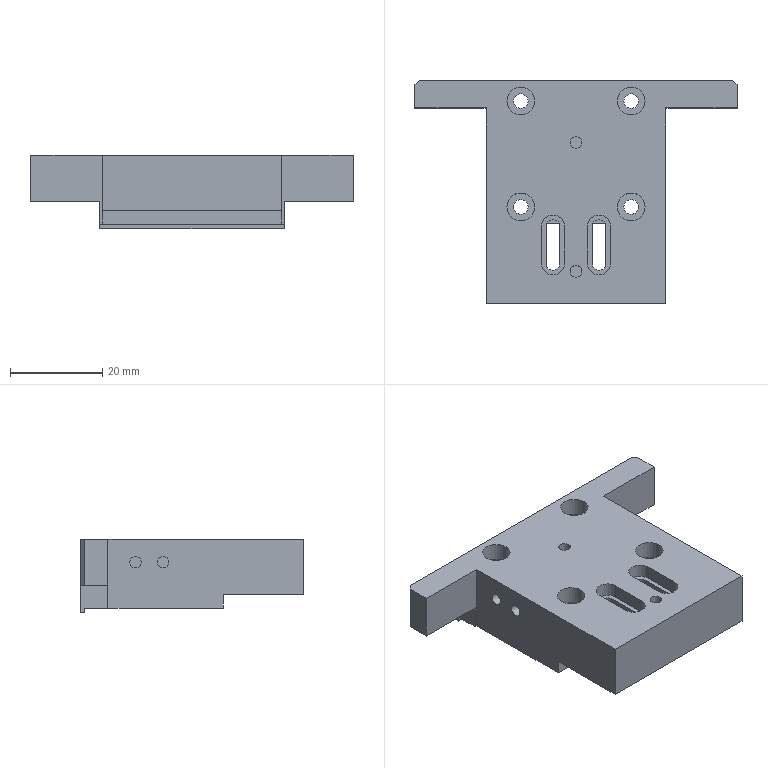NC program | NX | posted with a generic post | part box 70 x 48.5 x 16 mm
Whole program:
N10 G17 G21 G94 G90
(ADAPTIVE_MILLING , TOOL : D10)
N12 T15 M6
N14 G54
N16 G17 G0 G90 X-47.709 Y16.813 S9500 M3
N18 G43 Z30. H15
N20 Z-13.
N22 G94 G1 Z-16. F1000.
N24 X-46.929 Y16.533 F3000.
N26 X-46.14 Y16.277
N28 G3 X-45.062 Y16.813 R1.017
N30 X-44.301 Y19.876 R8.317
N32 X-44.012 Y26.743 R102.535
N34 G2 X-41.241 Y30.87 R6.021
N36 X-35.489 Y32.81 R13.418
N38 X-26.879 Y33.215 R73.526
N40 G1 X-25.629 Y33.223
N42 X-24.129 Y33.229
N44 X-22.004 Y33.234
N46 X-18.379 Y33.237
N48 X-7.254 Y33.239
N50 X36.996 Y33.238
N52 G2 X41.327 Y30.839 R5.654
N54 X43.446 Y25.422 R12.093
N56 X43.953 Y17.196 R56.705
N58 G1 X43.965 Y16.071
N60 X43.973 Y14.821
N62 X43.98 Y13.196
N64 X43.984 Y10.946
N66 X43.988 Y7.071
N68 X43.989 Y-5.304
N70 Y-26.304
N72 X43.987 Y-26.429
N74 X43.979 Y-26.554
N76 X43.968 Y-26.679
N78 G2 X41.138 Y-30.902 R6.019
N80 X35.747 Y-32.764 R13.208
N82 X27.515 Y-33.208 R64.336
N84 G1 X26.39 Y-33.217
N86 X25.015 Y-33.225
N88 X23.14 Y-33.231
N90 X20.39 Y-33.236
N92 X15.015 Y-33.238
N94 X-36.985
N96 G2 X-41.244 Y-30.948 R5.599
N98 X-43.423 Y-25.559 R11.833
N100 X-43.945 Y-17.834 R51.212
N102 G1 X-43.955 Y-17.084
N104 X-43.965 Y-16.084
N106 X-43.973 Y-14.834
N108 X-43.979 Y-13.334
N110 X-43.984 Y-10.959
N112 X-43.987 Y-7.209
N114 X-43.988 Y5.166
N116 Y13.041
N118 X-43.987 Y13.166
N120 X-43.985 Y13.291
N122 X-43.978 Y13.541
N124 X-43.973 Y13.666
N126 G2 X-43.376 Y19.509 R225.274
N128 X-43.06 Y24.247 R228.864
N130 X-39.015 Y29.825 R8.008
N132 X-32.603 Y31.779 R16.651
N134 X-22.242 Y32.208 R94.118
N136 G1 X-20.867 Y32.215
N138 X-18.867 Y32.221
N140 X-15.867 Y32.225
N142 X-10.117 Y32.227
N144 X33.883 Y32.228
N146 X34.133 Y32.225
N148 G2 X40.324 Y28.549 R7.632
N150 X42.447 Y22.328 R15.339
N152 X42.937 Y13.723 R67.586
N154 G1 X42.949 Y12.599
N156 X42.958 Y11.349
N158 X42.966 Y9.599
N160 X42.972 Y7.599
N162 X42.976 Y4.474
N164 X42.978 Y-2.151
N166 Y-23.151
N168 X42.977 Y-23.276
N170 X42.974 Y-23.401
N172 X42.969 Y-23.526
N174 X42.963 Y-23.651
N176 X42.954 Y-23.776
N178 G2 X39.07 Y-29.718 R7.757
N180 X32.438 Y-31.78 R16.302
N182 X22.827 Y-32.203 R89.297
N184 G1 X21.577 Y-32.211
N186 X19.827 Y-32.218
N188 X17.327 Y-32.223
N190 X13.327 Y-32.226
N192 X1.452 Y-32.227
N194 X-33.923 Y-32.228
N196 G2 X-40.279 Y-28.622 R7.603
N198 X-42.474 Y-22.167 R15.439
N200 X-42.947 Y-12.81 R76.871
N202 G1 X-42.957 Y-11.56
N204 X-42.965 Y-10.06
N206 X-42.971 Y-8.06
N208 X-42.975 Y-5.185
N210 X-42.977 Y0.315
N212 X-42.978 Y10.69
N214 G2 X-42.495 Y18.172 R98.901
N216 X-42.111 Y22.402 R47.689
N218 X-37.061 Y28.871 R9.339
N220 X-29.987 Y30.799 R19.765
N222 X-19.499 Y31.195 R111.929
N224 G1 X-17.874 Y31.203
N226 X-15.874 Y31.209
N228 X-12.999 Y31.214
N230 X-7.749 Y31.216
N232 X31.251 Y31.217
N234 X31.501 Y31.215
N236 G2 X39.448 Y26.438 R8.937
N238 X41.492 Y19.532 R18.317
N240 X41.939 Y9.422 R96.25
N242 G1 X41.948 Y8.047
N244 X41.956 Y6.297
N246 X41.962 Y3.922
N248 X41.965 Y0.297
N250 X41.967 Y-7.703
N252 Y-20.453
N254 G2 X37.233 Y-28.675 R8.948
N256 X30.331 Y-30.734 R18.449
N258 X20.472 Y-31.186 R90.512
N260 G1 X19.097 Y-31.196
N262 X17.347 Y-31.204
N264 X15.347 Y-31.21
N266 X12.222 Y-31.214
N268 X6.222 Y-31.216
N270 X-31.278 Y-31.217
N272 G2 X-39.463 Y-26.418 R8.968
N274 X-41.494 Y-19.508 R18.373
N276 X-41.946 Y-8.398 R104.034
N278 X-41.914 Y11.601 R861.952
N280 X-41.274 Y20.2 R123.382
N282 X-40.051 Y23.726 R11.366
N284 X-39.374 Y25.855 R5.518
N286 X-36.486 Y28.693 R10.78
N288 X-33.965 Y29.35 R5.988
N290 X-19.247 Y30.17 R121.248
N292 G1 X-17.872 Y30.181
N294 X-16.497 Y30.189
N296 X-14.497 Y30.196
N298 X-11.747 Y30.202
N300 X-7.497 Y30.205
N302 X3.878 Y30.206
N304 X28.878
N306 X29.128 Y30.205
N308 X29.503 Y30.199
N310 X29.628 Y30.196
N312 X29.877 Y30.187
N314 X30.002 Y30.181
N316 G2 X33.769 Y29.358 R13.209
N318 X36.605 Y28.624 R6.009
N320 X39.443 Y25.736 R10.78
N322 X40.111 Y23.091 R6.229
N324 X40.928 Y7.497 R131.705
N326 G1 X40.937 Y6.122
N328 X40.945 Y4.247
N330 X40.95 Y1.747
N332 X40.954 Y-2.003
N334 X40.956 Y-9.753
N336 Y-18.128
N338 G2 X39.472 Y-24.103 R10.532
N340 X33.706 Y-28.493 R11.431
N342 X26.117 Y-29.925 R27.15
N344 X12.247 Y-30.2 R225.837
N346 G1 X8.747 Y-30.204
N348 X1.497 Y-30.206
N350 X-28.878
N352 X-29.128 Y-30.205
N354 X-29.503 Y-30.199
N356 X-29.753 Y-30.192
N358 G2 X-38.298 Y-24.998 R9.757
N360 X-40.431 Y-17.857 R19.285
N362 X-40.925 Y-7.124 R97.507
N364 X-40.891 Y11. R651.393
N366 X-40.338 Y18.601 R79.735
N368 G1 X-40.293 Y18.847
N370 X-40.269 Y18.97
N372 X-40.217 Y19.214
N374 X-40.19 Y19.336
N376 X-40.162 Y19.458
N378 X-40.133 Y19.58
N380 X-40.108 Y19.702
N382 X-40.1 Y19.757
N384 Y23.215
N386 X-40.095 Y23.284
N388 X-40.014 Y23.904
N390 X-39.97 Y24.271
N392 X-39.9 Y24.634
N394 G2 X-38.582 Y26.881 R6.064
N396 X-36.486 Y28.693 R11.569
N398 X-33.965 Y29.35 R6.064
N400 G1 X33.91
N402 X34.582 Y29.278
N404 X35.251 Y29.185
N406 G2 X37.631 Y27.832 R5.972
N408 X39.443 Y25.736 R11.569
N410 X40.1 Y23.215 R6.064
N412 G1 Y18.285
N414 X40.095 Y18.216
N416 G3 X39.905 Y12.348 R48.092
N418 G1 X39.914 Y10.848
N420 X39.922 Y9.723
N422 X39.923 Y8.973
N424 X39.931 Y7.723
N426 X39.934 Y6.473
N428 X39.938 Y5.723
N430 X39.94 Y4.723
N432 X39.941 Y3.973
N434 X39.944 Y3.348
N436 X39.947 Y1.973
N438 Y0.848
N440 X39.95 Y0.098
N442 Y-0.902
N444 X39.952 Y-1.652
N446 X39.953 Y-2.152
N448 X39.952 Y-3.402
N450 X39.954 Y-4.152
N452 Y-5.152
N454 X39.953 Y-5.527
N456 G2 X39.91 Y-17.651 R472.767
N458 X34.043 Y-26.619 R10.481
N460 X26.743 Y-28.669 R21.093
N462 X21.134 Y-29.073 R79.695
N464 X19.465 Y-29.35 R8.967
N466 G1 X-19.465
N468 X-19.534 Y-29.345
N470 G3 X-28.282 Y-29.177 R880.45
N472 G2 X-37.37 Y-23.294 R10.494
N474 X-39.404 Y-16.117 R21.106
N476 X-39.913 Y-5.009 R101.039
N478 X-39.853 Y10.989 R438.887
N480 G1 X-39.828 Y11.614
N482 X-39.8 Y12.238
N484 X-39.768 Y12.862
N486 X-39.727 Y13.611
N488 X-39.683 Y14.36
N490 X-39.658 Y14.734
N492 X-39.641 Y14.984
N494 X-39.611 Y15.357
N496 X-39.6 Y15.482
N498 X-39.576 Y15.731
N500 X-39.57 Y15.856
N502 X-39.578 Y15.98
N504 G3 X-39.935 Y16.999 R13.065
N506 G2 X-40.1 Y19.785 R13.155
N508 G3 X-41.518 Y20.693 R1.002
N510 X-42.103 Y19.958 Z-15.952 R1.133
N512 G1 X-42.461 Y18.993 Z-15.9
N514 X-43.254 Y16.838
N516 X-43.282 Y16.603
N518 Y-7.772
N520 G3 X-42.499 Y-16.452 R48.938
N522 G1 X-41.904 Y-19.644
N524 G3 X-40.018 Y-24.779 R21.419
N526 X-38.27 Y-27.357 R16.875
N528 G1 X-37.147 Y-28.694
N530 G3 X-34.339 Y-30.712 R9.317
N532 X-31.049 Y-31.832 R16.943
N534 G1 X-30.131 Y-31.99
N536 X-29.206 Y-32.09
N538 X-22.716 Y-32.527
N540 X-22.494 Y-32.514
N542 X-22.278 Y-32.458
N544 X-20.512 Y-31.753
N546 X-19.821 Y-31.483 Z-15.937
N548 X-19.14 Y-31.188 Z-15.974
N550 X-18.943 Y-31.024 Z-15.987
N552 X-18.789 Y-30.819 Z-16.
N554 G3 X-19.534 Y-29.345 R1.002
N556 G2 X-21.835 Y-28.844 R8.931
N558 G3 X-26.673 Y-28.287 R34.892
N560 G2 X-36.536 Y-21.471 R11.375
N562 X-38.493 Y-13.498 R24.43
N564 X-38.914 Y-1.135 R140.043
N566 X-38.689 Y14.236 R266.321
N568 G3 X-38.868 Y14.985 R1.552
N570 G2 X-39.635 Y16.226 R3.82
N572 G3 X-41.233 Y16.582 R1.003
N574 X-41.572 Y15.742 Z-15.953 R1.153
N576 G1 X-41.669 Y14.68 Z-15.9
N578 X-41.869 Y12.471
N580 X-42.037 Y10.26
N582 X-42.074 Y8.601
N584 X-41.959 Y-8.903
N586 G3 X-41.186 Y-16.328 R38.92
N588 X-40.326 Y-19.969 R37.817
N590 X-38.826 Y-23.932 R37.833
N592 X-36.068 Y-27.405 R9.681
N594 G1 X-33.706 Y-29.25
N596 G3 X-30.818 Y-30.682 R11.048
N598 G1 X-30.222 Y-30.862
N600 X-29.619 Y-31.021
N602 X-24.182 Y-32.284
N604 G3 X-23.509 Y-32.204 R1.038
N606 G1 X-21.949 Y-31.426
N608 X-21.363 Y-31.139 Z-15.933
N610 X-20.788 Y-30.83 Z-15.965
N612 G3 X-20.411 Y-30.263 Z-16. R1.038
N614 X-21. Y-29.102 R1.005
N616 X-23.133 Y-28.172 R132.375
N618 X-27.149 Y-27.24 R75.523
N620 G2 X-35.564 Y-20.024 R12.312
N622 X-37.483 Y-11.909 R26.073
N624 X-37.898 Y-0.045 R141.135
N626 X-37.765 Y12.703 R430.215
N628 G3 X-38.056 Y14.156 R2.927
N630 X-38.649 Y14.699 R7.77
N632 G1 X-38.877 Y14.997
N634 G3 X-40.169 Y15.255 R1.005
N636 X-40.674 Y14.427 Z-15.95 R1.036
N638 G1 X-40.811 Y13.447 Z-15.9
N640 X-40.977 Y12.274
N642 X-41.127 Y11.099
N644 Y-4.526
N646 G3 X-40.408 Y-13.216 R53.484
N648 G1 X-40.118 Y-14.961
N650 X-39.78 Y-16.697
N652 G3 X-38.205 Y-21.639 R29.466
N654 X-34.556 Y-26.609 R14.315
N656 X-30.988 Y-29.033 R14.286
N658 G1 X-30.421 Y-29.277
N660 X-29.846 Y-29.502
N662 X-26.002 Y-30.874
N664 X-25.751 Y-30.925
N666 X-25.494 Y-30.918
N668 X-23.645 Y-30.595
N670 X-22.4 Y-30.367 Z-15.963
N672 G3 X-21.845 Y-29.912 Z-16. R1.03
N674 X-22.105 Y-28.624 R1.005
N676 X-24.933 Y-27.066 R8.103
N678 G2 X-30.281 Y-24.407 R18.717
N680 X-35.245 Y-16.922 R14.883
N682 X-36.655 Y-7.931 R36.966
N684 X-36.803 Y10.565 R263.542
N686 G3 X-37.153 Y13.401 R8.137
N688 X-37.605 Y13.876 R1.523
N690 G1 X-38.299 Y14.408
N692 G3 X-39.413 Y14.478 R1.01
N694 X-39.907 Y13.722 Z-15.953 R1.047
N696 G1 X-40.123 Y12.679 Z-15.9
N698 X-40.544 Y10.613
N700 X-40.553 Y6.032
N702 X-40.537 Y1.451
N704 G3 X-39.723 Y-9.434 R95.319
N706 G1 X-39.106 Y-13.973
N708 G3 X-37.645 Y-19.343 R25.977
N710 X-35.655 Y-23.004 R20.14
N712 X-30.83 Y-27.795 R16.869
N714 G1 X-26.697 Y-30.342
N716 G3 X-25.96 Y-30.466 R1.028
N718 G1 X-24.306 Y-30.105
N720 X-23.665 Y-29.97 Z-15.933
N722 X-23.03 Y-29.811 Z-15.966
N724 G3 X-22.527 Y-29.358 Z-16. R1.038
N726 X-22.799 Y-28.092 R1.006
N728 G1 X-23.777 Y-27.196
N730 G3 X-27.195 Y-25.123 R57.228
N732 G2 X-34.193 Y-15.862 R16.125
N734 X-35.635 Y-6.623 R38.708
N736 X-35.831 Y9.373 R277.92
N738 G3 X-36.297 Y12.823 R10.063
N740 X-36.903 Y13.565 R1.361
N742 G1 X-37.486 Y13.807
N744 X-37.594 Y13.869
N746 G3 X-38.587 Y13.873 R1.014
N748 X-39.088 Y13.149 Z-15.955 R1.05
N750 G1 X-39.351 Y12.092 Z-15.9
N752 X-39.838 Y10.102
N754 G3 X-39.674 Y3.232 R176.229
N756 G1 X-39.523 Y0.99
N758 X-39.321 Y-1.248
N760 X-38.838 Y-5.884
N762 X-38.333 Y-10.518
N764 G3 X-36.794 Y-17.739 R45.792
N766 G1 X-36.235 Y-19.551
N768 G3 X-33.133 Y-24.128 R11.365
N770 X-29.471 Y-27.339 R59.965
N772 G1 X-27.571 Y-28.867
N774 G3 X-27.021 Y-29.084 R1.048
N776 G1 X-25.209 Y-29.223
N778 X-23.947 Y-29.308 Z-15.963
N780 G3 X-23.297 Y-29.003 Z-16. R1.03
N782 X-23.225 Y-27.702 R1.005
N784 X-25.622 Y-25.254 R10.406
N786 G2 X-30.768 Y-20.02 R22.239
N788 X-33.968 Y-11.413 R22.175
N790 X-34.804 Y-0.08 R77.639
N792 G3 X-34.883 Y9.169 R726.815
N794 X-35.596 Y12.697 R8.841
N796 X-36.384 Y13.35 R1.198
N798 G1 X-36.962 Y13.59
N800 G3 X-38.061 Y13.363 R1.01
N802 X-38.336 Y12.504 Z-15.953 R1.047
N804 G1 X-38.267 Y11.44 Z-15.9
N806 X-38.126 Y9.243
N808 X-38.133 Y4.244
N810 X-38.115 Y-0.755
N812 G3 X-37.366 Y-9.449 R66.209
N814 G1 X-36.764 Y-13.275
N816 G3 X-34.159 Y-20.108 R20.712
N818 X-31.34 Y-24.207 R30.391
N820 G1 X-28.221 Y-28.02
N822 G3 X-27.435 Y-28.387 R1.016
N824 G1 X-25.883 Y-28.369
N826 X-25.221 Y-28.366 Z-15.933
N828 X-24.561 Y-28.339 Z-15.966
N830 G3 X-23.984 Y-28.01 Z-16. R1.039
N832 X-23.874 Y-26.855 R1.007
N834 X-25.777 Y-24.23 R8.703
N836 G2 X-30.463 Y-18.093 R26.855
N838 X-33.218 Y-8.537 R27.604
N840 X-33.812 Y4.567 R113.274
N842 G3 X-34.166 Y10.549 R36.42
N844 X-35.163 Y12.943 R5.045
N846 X-36.251 Y13.315 R1.714
N848 G1 X-36.372 Y13.347
N850 G3 X-37.335 Y13.091 R1.014
N852 X-37.627 Y12.254 Z-15.954 R1.049
N854 G1 X-37.597 Y11.17 Z-15.9
N856 X-37.536 Y9.
N858 X-37.523 Y4.002
N860 G3 X-37.071 Y-2.221 R61.943
N862 G1 X-36.559 Y-6.355
N864 X-36.027 Y-10.487
N866 G3 X-34.632 Y-16.127 R30.46
N868 X-32.797 Y-20.026 R25.448
N870 X-30.679 Y-23.407 R46.623
N872 G1 X-28.539 Y-26.505
N874 G3 X-28.043 Y-26.882 R1.044
N876 G1 X-26.346 Y-27.468
N878 X-25.147 Y-27.87 Z-15.963
N880 G3 X-24.441 Y-27.74 Z-16. R1.03
N882 X-24.039 Y-26.505 R1.006
N884 X-26.338 Y-22.441 R13.899
N886 G2 X-32.05 Y-8.632 R28.04
N888 X-32.781 Y3.587 R95.073
N890 G3 X-33.191 Y9.817 R42.062
N892 X-34.397 Y12.794 R6.242
N894 X-35.035 Y13.155 R1.363
N896 G1 X-35.778 Y13.252
N898 G3 X-36.698 Y12.875 R1.014
N900 X-36.911 Y12.08 Z-15.958 R1.182
N902 G1 X-36.925 Y10.923 Z-15.9
N904 X-36.943 Y8.906
N906 X-35.388 Y-6.642
N908 G3 X-33.747 Y-15.027 R46.766
N910 X-30.274 Y-22.223 R27.113
N912 G1 X-28.746 Y-24.47
N914 X-28.533 Y-24.697
N916 X-26.887 Y-25.977
N918 X-26.37 Y-26.386 Z-15.933
N920 X-25.837 Y-26.775 Z-15.966
N922 G3 X-25.178 Y-26.875 Z-16. R1.039
N924 X-24.4 Y-25.634 R1.004
N926 X-25.566 Y-22.351 R8.087
N928 G2 X-28.955 Y-15.809 R54.922
N930 X-31.318 Y-5.36 R37.445
N932 X-31.812 Y4.751 R171.366
N934 G3 X-32.55 Y10.564 R24.225
N936 X-33.882 Y12.929 R4.958
N938 X-35.034 Y13.155 R1.836
N940 G1 X-35.158 Y13.171
N942 G3 X-36.094 Y12.772 R1.011
N944 X-36.291 Y11.995 Z-15.959 R1.2
N946 G1 X-36.306 Y10.814 Z-15.9
N948 X-36.323 Y8.824
N950 X-35.82 Y4.48
N952 X-35.262 Y0.143
N954 X-34.939 Y-2.02
N956 X-34.597 Y-4.179
N958 X-34.009 Y-7.721
N960 X-33.404 Y-11.261
N962 G3 X-32.1 Y-16.141 R32.335
N964 G1 X-31.546 Y-17.531
N966 X-28.864 Y-23.717
N968 G3 X-28.517 Y-24.14 R1.057
N970 G1 X-27.002 Y-25.192
N972 X-25.953 Y-25.907 Z-15.964
N974 G3 X-25.242 Y-25.976 Z-16. R1.031
N976 X-24.517 Y-24.881 R1.005
N978 X-24.847 Y-22.742 R12.416
N980 X-26.913 Y-17.919 R49.356
N982 G2 X-30.373 Y-3.661 R41.697
N984 X-30.909 Y5.949 R980.161
N986 G3 X-32.036 Y11.306 R16.701
N988 X-33.393 Y13.052 R3.547
N990 X-34.51 Y13.15 R2.97
N992 X-35.451 Y12.62 R1.112
N994 X-35.534 Y11.605 Z-15.948 R1.228
N996 G1 X-35.309 Y10.684 Z-15.9
N998 X-27.098 Y-22.999
N1000 X-26.918 Y-23.749 Z-15.939
N1002 X-26.723 Y-24.496 Z-15.977
N1004 X-26.614 Y-24.696 Z-15.989
N1006 X-26.472 Y-24.874 Z-16.
N1008 G3 X-24.6 Y-24.09 R1.101
N1010 X-25.347 Y-19.564 R10.477
N1012 G2 X-28.01 Y-11.497 R77.245
N1014 X-29.539 Y-0.118 R60.408
N1016 G3 X-30.218 Y7.849 R77.603
N1018 X-31.825 Y12.277 R10.665
N1020 X-33.019 Y13.15 R1.841
N1022 G1 X-33.769
N1024 G3 X-34.721 Y12.602 R1.112
N1026 X-34.796 Y11.611 Z-15.949 R1.243
N1028 G1 X-34.576 Y10.66 Z-15.9
N1030 X-27.098 Y-21.556
N1032 X-26.732 Y-23.097 Z-15.979
N1034 X-26.638 Y-23.282 Z-15.99
N1036 X-26.518 Y-23.451 Z-16.
N1038 G3 X-24.6 Y-22.715 R1.101
N1040 X-25.314 Y-17.294 R14.763
N1042 G2 X-27.932 Y-5.982 R69.665
N1044 X-28.78 Y3.729 R207.728
N1046 G3 X-29.97 Y10.227 R25.791
N1048 X-31.688 Y12.942 R6.24
N1050 X-32.259 Y13.15 R1.973
N1052 G1 X-33.134
N1054 G3 X-34.084 Y12.603 R1.112
N1056 X-34.164 Y11.617 Z-15.949 R1.246
N1058 G1 X-33.948 Y10.66 Z-15.9
N1060 X-27.098 Y-19.762
N1062 X-26.923 Y-20.57 Z-15.941
N1064 X-26.722 Y-21.372 Z-15.983
N1066 X-26.642 Y-21.525 Z-15.991
N1068 X-26.546 Y-21.669 Z-16.
N1070 G3 X-24.6 Y-20.965 R1.101
N1072 X-24.764 Y-16.85 R24.552
N1074 X-26.334 Y-9.261 R900.587
N1076 G2 X-27.625 Y1.909 R112.257
N1078 G3 X-28.77 Y9.181 R36.952
N1080 X-30.701 Y12.778 R8.267
N1082 X-31.47 Y13.15 R1.356
N1084 G1 X-32.345
N1086 G3 X-33.295 Y12.605 R1.112
N1088 X-33.378 Y11.623 Z-15.949 R1.248
N1090 G1 X-33.168 Y10.66 Z-15.9
N1092 X-27.099 Y-17.213
N1094 X-26.924 Y-18.035 Z-15.942
N1096 X-26.73 Y-18.852 Z-15.984
N1098 X-26.576 Y-19.13 Z-16.
N1100 G3 X-24.6 Y-18.465 R1.101
N1102 X-24.736 Y-13.346 R42.345
N1104 G2 X-26.116 Y-3.317 R264.915
N1106 G3 X-27.148 Y5.999 R148.189
N1108 X-29.002 Y11.669 R16.291
N1110 X-30.369 Y13.088 R3.362
N1112 X-31.519 Y13.15 R4.342
N1114 X-32.469 Y12.605 R1.112
N1116 X-32.553 Y11.626 Z-15.949 R1.25
N1118 G1 X-32.346 Y10.66 Z-15.9
N1120 X-27.099 Y-13.813
N1122 X-26.924 Y-14.642 Z-15.942
N1124 X-26.733 Y-15.467 Z-15.985
N1126 X-26.591 Y-15.736 Z-16.
N1128 G3 X-24.6 Y-15.09 R1.101
N1130 X-24.67 Y-8.342 R112.507
N1132 X-25.996 Y4.714 R251.025
N1134 X-27.753 Y10.944 R20.967
N1136 X-29.348 Y12.997 R5.591
N1138 G1 X-29.823 Y13.15
N1140 X-30.698
N1142 G3 X-31.649 Y12.602 R1.112
N1144 X-31.726 Y11.613 Z-15.949 R1.244
N1146 G1 X-31.508 Y10.66 Z-15.9
N1148 X-27.1 Y-8.534
N1150 X-26.745 Y-10.046 Z-15.978
N1152 X-26.657 Y-10.25 Z-15.989
N1154 X-26.532 Y-10.435 Z-16.
N1156 G3 X-24.6 Y-9.715 R1.101
N1158 X-24.635 Y0.409 R459.984
N1160 X-26.166 Y9.249 R33.
N1162 X-28.227 Y12.779 R8.872
N1164 X-29. Y13.15 R1.377
N1166 G1 X-29.875
N1168 G3 X-30.84 Y12.577 R1.112
N1170 X-30.887 Y11.607 Z-15.95 R1.149
N1172 G1 X-30.571 Y10.662 Z-15.9
N1174 X-27.102 Y0.263
N1176 X-26.9 Y-0.358 Z-15.933
N1178 X-26.676 Y-0.973 Z-15.965
N1180 G3 X-26.19 Y-1.45 Z-16. R1.145
N1182 X-24.6 Y-0.465 R1.102
N1184 X-24.643 Y5.908 R137.156
N1186 X-26.86 Y12.201 R12.706
N1188 X-28.13 Y13.147 R2.108
N1190 G1 X-28.152 Y13.15
N1192 X-29.027
N1194 G3 X-30.017 Y12.53 R1.111
N1196 X-29.938 Y11.407 Z-15.941 R1.199
N1198 G1 X-29.579 Y10.664 Z-15.9
N1200 X-27.106 Y5.541
N1202 X-26.863 Y5.032 Z-15.928
N1204 X-26.603 Y4.531 Z-15.957
N1206 G3 X-25.887 Y4.076 Z-16. R1.128
N1208 X-24.6 Y5.16 R1.103
N1210 X-24.67 Y8.656 R30.698
N1212 X-26.697 Y12.858 R7.224
N1214 X-27.374 Y13.15 R1.376
N1216 G1 X-28.249
N1218 G3 X-29.185 Y11.473 R1.102
N1220 G1 X-26.637 Y7.333
N1222 G3 X-24.6 Y7.91 R1.101
N1224 X-24.73 Y10.524 R11.603
N1226 X-26.15 Y12.965 R4.477
N1228 X-27.426 Y13.15 R2.257
N1230 X-28.333 Y11.428 R1.101
N1232 G1 X-26.607 Y8.912
N1234 G3 X-24.6 Y9.535 R1.101
N1236 X-24.757 Y11.643 R6.762
N1238 X-25.86 Y13.086 R2.159
N1240 X-26.764 Y13.15 R3.32
N1242 X-27.606 Y11.342 R1.101
N1244 G1 X-26.542 Y10.077
N1246 G3 X-24.6 Y10.785 R1.101
N1248 X-24.91 Y12.602 R3.209
N1250 X-26.156 Y13.15 R1.253
N1252 X-26.98 Y11.321 R1.101
N1254 G1 X-26.694 Y10.996
N1256 X-26.396 Y10.683
N1258 G3 X-24.6 Y11.535 R1.101
N1260 X-24.742 Y12.619 R2.221
N1262 X-25.788 Y13.15 R1.124
N1264 X-25.906 Y11.087 R1.036
N1266 X-24.636 Y12.362 R1.118
N1268 X-26.282 Y12.834 R1.016
N1270 X-26.599 Y12.228 R1.038
N1272 G1 X-26.679 Y11.629
N1274 X-26.894 Y10.079 Z-15.922
N1276 X-26.963 Y9.874 Z-15.911
N1278 X-27.073 Y9.687 Z-15.9
N1280 G2 X-27.866 Y9.296 R1.015
N1282 G1 X-31.076 Y9.309
N1284 G2 X-35.285 Y9.928 R19.778
N1286 G1 X-37.025 Y10.376
N1288 X-38.758 Y10.849
N1290 G2 X-40.518 Y11.948 R4.68
N1292 X-43.051 Y16.165 R9.849
N1294 X-43.338 Y18.616 R7.841
N1296 G1 X-43.117 Y23.611
N1298 G2 X-42.685 Y26.052 R9.739
N1300 X-42.132 Y27.504 R7.816
N1302 X-41.19 Y28.733 R5.211
N1304 G1 X-39.526 Y30.307
N1306 G2 X-35.927 Y32.048 R8.286
N1308 X-32.971 Y32.377 R18.01
N1310 G1 X10.768 Y33.623
N1312 G2 X28.218 Y32.974 R133.996
N1314 G1 X34.435 Y32.332
N1316 G2 X38.985 Y30.664 R9.907
N1318 X40.904 Y29.115 R10.775
N1320 X42.78 Y25.985 R8.018
N1322 X43.09 Y24.181 R7.546
N1324 G1 X43.228 Y21.026
N1326 G2 X42.801 Y20.161 R1.014
N1328 G1 X42.648 Y20.054
N1330 X41.007 Y18.911 Z-16.
N1332 X40.668 Y18.675
N1334 X40.338 Y18.428
N1336 G3 X40.047 Y17.844 R1.04
N1338 G2 X39.594 Y16.046 R5.611
N1340 G3 X39.031 Y11.09 R21.688
N1342 X38.96 Y-8.784 R950.405
N1344 G2 X38.868 Y-16.407 R127.15
N1346 X32.629 Y-25.576 R10.999
N1348 X24.704 Y-27.696 R22.829
N1350 G3 X23.097 Y-27.912 R11.318
N1352 X21.986 Y-28.693 R15.654
N1354 G1 X20.946 Y-29.124
N1356 G3 X20.576 Y-30.706 R1.003
N1358 X21.413 Y-31.063 Z-15.953 R1.151
N1360 G1 X22.469 Y-31.178 Z-15.9
N1362 X24.61 Y-31.404
N1364 X24.843 Y-31.374
N1366 X27.066 Y-30.82
N1368 X29.283 Y-30.249
N1370 G3 X34.411 Y-28.104 R23.196
N1372 X38.496 Y-24.856 R19.734
N1374 X41.441 Y-19.293 R11.787
N1376 X41.902 Y-15.591 R21.861
N1378 G1 X42.938 Y13.337
N1380 X42.916 Y13.567
N1382 X42.849 Y13.788
N1384 X42.061 Y15.518
N1386 X41.795 Y16.115 Z-15.933
N1388 X41.505 Y16.701 Z-15.965
N1390 G3 X40.955 Y17.098 Z-16. R1.038
N1392 X39.756 Y16.519 R1.005
N1394 G2 X38.981 Y14.865 R27.359
N1396 G3 X38.152 Y9.952 R17.53
N1398 X37.966 Y-3.545 R288.54
N1400 G2 X37.882 Y-14.543 R287.113
N1402 X31.252 Y-24.548 R11.516
N1404 X25.307 Y-26.41 R23.116
N1406 G3 X23.895 Y-26.885 R4.265
N1408 X23.051 Y-27.899 R29.656
N1410 G1 X22.853 Y-28.051
N1412 G3 X22.89 Y-29.665 R1.003
N1414 X23.815 Y-29.798 Z-15.952 R1.135
N1416 G1 X24.835 Y-29.624 Z-15.9
N1418 X27.199 Y-29.216
N1420 X29.612 Y-28.573
N1422 G3 X35.555 Y-25.283 R16.132
N1424 G1 X37.327 Y-23.712
N1426 G3 X39.691 Y-19.955 R10.004
N1428 X40.748 Y-15.122 R15.825
N1430 X41.032 Y-10.141 R88.906
N1432 G1 X41.624 Y11.748
N1434 X41.615 Y11.913
N1436 X41.314 Y14.058
N1438 X41.23 Y14.703 Z-15.933
N1440 X41.119 Y15.345 Z-15.965
N1442 G3 X40.698 Y15.884 Z-16. R1.038
N1444 X39.374 Y15.645 R1.005
N1446 X37.616 Y11.704 R7.633
N1448 X37.034 Y3.484 R51.535
N1450 G1 X37.021 Y2.609
N1452 X37.011 Y1.609
N1454 X36.998 Y-0.016
N1456 X36.989 Y-1.641
N1458 X36.982 Y-3.391
N1460 X36.976 Y-4.141
N1462 X36.972 Y-5.141
N1464 X36.971 Y-6.016
N1466 X36.966 Y-7.016
N1468 Y-8.016
N1470 Y-8.391
N1472 X36.96 Y-9.516
N1474 X36.949 Y-10.891
N1476 X36.94 Y-11.516
N1478 G2 X35.828 Y-17.622 R15.589
N1480 X29.494 Y-23.727 R12.251
N1482 X25.289 Y-25.324 R97.905
N1484 G3 X24.202 Y-26.112 R2.007
N1486 G2 X23.722 Y-27.054 R3.515
N1488 G3 X23.795 Y-28.355 R1.005
N1490 X24.722 Y-28.646 Z-15.949 R1.036
N1492 G1 X25.704 Y-28.539 Z-15.9
N1494 X27.847 Y-28.298
N1496 X28.069 Y-28.218
N1498 X30.408 Y-27.033
N1500 G3 X33.933 Y-24.623 R24.437
N1502 X36.946 Y-21.822 R30.143
N1504 X39.017 Y-17.905 R9.395
N1506 X39.757 Y-13.618 R21.822
N1508 G1 X40.111 Y-8.007
N1510 X40.406 Y-2.392
N1512 X41.015 Y11.047
N1514 X40.709 Y13.251
N1516 X40.622 Y13.902 Z-15.933
N1518 X40.511 Y14.549 Z-15.966
N1520 G3 X40.101 Y15.083 Z-16. R1.039
N1522 X38.766 Y14.851 R1.005
N1524 X37.762 Y13.643 R7.576
N1526 X36.461 Y8.975 R13.085
N1528 X36.026 Y-0.26 R87.209
N1530 G2 X35.878 Y-11.508 R358.48
N1532 X33.246 Y-18.922 R12.757
N1534 X27.998 Y-22.875 R15.039
N1536 G3 X24.834 Y-24.628 R17.933
N1538 X24.4 Y-25.634 R1.626
N1540 G1 X24.16 Y-26.212
N1542 G3 X24.585 Y-27.461 R1.005
N1544 X25.551 Y-27.484 Z-15.95 R1.037
N1546 G1 X26.473 Y-27.112 Z-15.9
N1548 X28.583 Y-26.256
N1550 X31.932 Y-24.137
N1552 G3 X34.674 Y-22.035 R26.265
N1554 X36.608 Y-19.462 R9.192
N1556 G1 X37.166 Y-18.352
N1558 X37.676 Y-17.218
N1560 G3 X38.563 Y-13.926 R16.39
N1562 G1 X38.769 Y-12.539
N1564 X38.919 Y-11.145
N1566 X40.702 Y10.628
N1568 X40.683 Y10.918
N1570 X40.284 Y12.79
N1572 X40.149 Y13.446 Z-15.934
N1574 X39.991 Y14.098 Z-15.967
N1576 G3 X39.573 Y14.591 Z-16. R1.041
N1578 X38.452 Y14.525 R1.01
N1580 X36.367 Y11.646 R5.302
N1582 X35.261 Y5.135 R24.788
N1584 X34.958 Y-8.36 R318.25
N1586 G2 X34.061 Y-14.391 R19.069
N1588 X28.871 Y-20.781 R13.123
N1590 G3 X25.359 Y-23.17 R55.109
N1592 X24.595 Y-24.284 R1.784
N1594 G1 X24.465 Y-25.276
N1596 G3 X24.954 Y-26.271 R1.01
N1598 X25.858 Y-26.327 Z-15.953 R1.047
N1600 G1 X26.868 Y-25.998 Z-15.9
N1602 X28.847 Y-25.344
N1604 G3 X30.438 Y-24.132 R7.906
N1606 G1 X32.537 Y-21.96
N1608 X34.62 Y-19.773
N1610 G3 X35.756 Y-18.061 R8.231
N1612 X36.944 Y-15.315 R30.359
N1614 X37.408 Y-13.383 R10.747
N1616 X38.067 Y-7.182 R69.041
N1618 G1 X39.028 Y9.793
N1620 X39.313 Y12.021
N1622 X39.402 Y12.669 Z-15.933
N1624 X39.465 Y13.321 Z-15.966
N1626 G3 X39.207 Y13.947 Z-16. R1.038
N1628 X37.857 Y14.069 R1.005
N1630 X36.42 Y12.769 R5.139
N1632 X34.81 Y8.335 R11.748
N1634 X34.109 Y-0.252 R56.681
N1636 G2 X33.852 Y-9.247 R197.98
N1638 X28.717 Y-19.166 R13.783
N1640 G3 X25.286 Y-22.074 R55.791
N1642 X24.6 Y-23.22 R2.061
N1644 G1 Y-24.215
N1646 X24.595 Y-24.284
N1648 G3 X25.335 Y-25.316 R1.007
N1650 X26.271 Y-25.092 Z-15.95 R1.037
N1652 G1 X27.072 Y-24.495 Z-15.9
N1654 X28.865 Y-23.163
N1656 X29.771 Y-22.69
N1658 X30.145 Y-22.417
N1660 X30.483 Y-22.101
N1662 X32.591 Y-19.793
N1664 G3 X36.686 Y-10.233 R17.058
N1666 G1 X38.653 Y9.495
N1668 X38.792 Y11.661
N1670 X38.84 Y12.323 Z-15.933
N1672 X38.863 Y12.987 Z-15.966
N1674 G3 X38.582 Y13.583 Z-16. R1.04
N1676 X37.486 Y13.807 R1.01
N1678 X35.321 Y11.834 R3.947
N1680 X33.66 Y6.234 R16.022
N1682 X33.068 Y-3.618 R89.001
N1684 G2 X32.56 Y-10.09 R39.493
N1686 X28.387 Y-17.637 R14.937
N1688 G3 X25.149 Y-20.936 R68.208
N1690 X24.6 Y-21.963 R2.138
N1692 G1 Y-23.338
N1694 G3 X25.324 Y-24.299 R1.007
N1696 X26.322 Y-24.054 Z-15.947 R1.111
N1698 G1 X27.086 Y-23.525 Z-15.9
N1700 X28.716 Y-22.395
N1702 X28.837 Y-22.29
N1704 X28.947 Y-22.173
N1706 X30.825 Y-19.676
N1708 X32.687 Y-17.166
N1710 G3 X34.453 Y-13.888 R17.96
N1712 X35.651 Y-9.714 R17.281
N1714 G1 X35.742 Y-9.099
N1716 X38.195 Y9.337
N1718 X38.329 Y11.446
N1720 X38.377 Y12.118 Z-15.934
N1722 X38.401 Y12.791 Z-15.967
N1724 G3 X38.137 Y13.374 Z-16. R1.042
N1726 X37.024 Y13.615 R1.01
N1728 X34.499 Y11.405 R4.409
N1730 X32.769 Y5.824 R16.381
N1732 X32.106 Y-3.146 R78.096
N1734 G2 X31.467 Y-9.353 R33.506
N1736 X27.466 Y-16.753 R17.277
N1738 G3 X24.778 Y-20.04 R31.586
N1740 X24.6 Y-20.553 R3.383
N1742 G1 Y-22.053
N1744 G3 X25.315 Y-23.012 R1.007
N1746 X26.314 Y-22.778 Z-15.947 R1.112
N1748 G1 X27.086 Y-22.257 Z-15.9
N1750 X27.93 Y-21.693
N1752 X28.763 Y-21.113
N1754 X28.947 Y-20.888
N1756 X30.591 Y-18.157
N1758 X32.216 Y-15.414
N1760 G3 X34.465 Y-9.123 R19.979
N1762 G1 X37.549 Y9.004
N1764 X37.591 Y10.069
N1766 X37.612 Y11.134
N1768 X37.633 Y11.824 Z-15.935
N1770 X37.635 Y12.514 Z-15.969
N1772 G3 X37.375 Y13.066 Z-16. R1.045
N1774 X36.384 Y13.35 R1.011
N1776 X34.258 Y11.904 R3.415
N1778 X32.152 Y6.87 R12.764
N1780 X31.227 Y-1.318 R50.315
N1782 G2 X30.554 Y-7.902 R42.9
N1784 X26.899 Y-15.498 R19.305
N1786 G3 X24.674 Y-18.665 R26.961
N1788 G1 X24.636 Y-18.783
N1790 X24.61 Y-18.906
N1792 X24.6 Y-18.975
N1794 Y-20.6
N1796 G3 X26.196 Y-21.581 R1.102
N1798 X26.805 Y-20.758 Z-15.947 R1.224
N1800 G1 X27.094 Y-19.862 Z-15.9
N1802 X37.009 Y10.914
N1804 X37.191 Y11.47 Z-15.929
N1806 X37.356 Y12.032 Z-15.959
N1808 G3 X37.183 Y12.823 Z-16. R1.13
N1810 X36.127 Y13.298 R1.112
N1812 X33.692 Y11.934 R3.441
N1814 X31.447 Y7.236 R11.901
N1816 X30.358 Y-0.173 R40.698
N1818 G2 X29.547 Y-6.993 R47.169
N1820 X26.102 Y-14.573 R22.583
N1822 G3 X24.666 Y-16.915 R30.554
N1824 G1 X24.63 Y-17.035
N1826 X24.606 Y-17.158
N1828 X24.6 Y-17.199
N1830 Y-19.074
N1832 G3 X26.195 Y-20.057 R1.102
N1834 X26.805 Y-19.233 Z-15.947 R1.224
N1836 G1 X27.094 Y-18.338 Z-15.9
N1838 X36.505 Y10.823
N1840 X36.69 Y11.39 Z-15.93
N1842 X36.86 Y11.961 Z-15.96
N1844 G3 X36.702 Y12.734 Z-16. R1.131
N1846 X35.631 Y13.233 R1.111
N1848 X32.892 Y11.72 R3.784
N1850 X30.499 Y6.679 R12.808
N1852 X29.34 Y-0.974 R47.899
N1854 G2 X27.701 Y-8.905 R29.532
N1856 X24.885 Y-14.477 R43.399
N1858 G3 X24.6 Y-15.211 R2.838
N1860 G1 Y-17.211
N1862 G3 X26.199 Y-18.192 R1.102
N1864 X26.805 Y-17.368 Z-15.947 R1.225
N1866 G1 X27.094 Y-16.47 Z-15.9
N1868 X35.834 Y10.725
N1870 X36.02 Y11.298 Z-15.93
N1872 X36.191 Y11.875 Z-15.96
N1874 G3 X36.04 Y12.638 Z-16. R1.132
N1876 X35.034 Y13.155 R1.112
N1878 X32.632 Y12.111 R3.294
N1880 X29.953 Y7.513 R11.032
N1882 X28.56 Y0.538 R36.135
N1884 G2 X26.966 Y-7.413 R38.737
N1886 X24.662 Y-12.676 R51.773
N1888 G1 X24.627 Y-12.796
N1890 X24.604 Y-12.919
N1892 X24.6 Y-12.95
N1894 Y-15.325
N1896 G3 X26.176 Y-16.317 R1.102
N1898 X26.803 Y-15.493 Z-15.947 R1.218
N1900 G1 X27.093 Y-14.611 Z-15.9
N1902 X35.417 Y10.665
N1904 X35.621 Y11.27 Z-15.932
N1906 X35.802 Y11.882 Z-15.964
N1908 G3 X35.679 Y12.581 Z-16. R1.142
N1910 X34.715 Y13.15 R1.112
N1912 X31.898 Y12.045 R3.563
N1914 X29.151 Y7.485 R11.315
N1916 X27.577 Y0.292 R39.381
N1918 G2 X24.643 Y-10.141 R38.035
N1920 G1 X24.614 Y-10.263
N1922 X24.6 Y-10.365
N1924 Y-12.99
N1926 G3 X26.16 Y-13.989 R1.102
N1928 X26.801 Y-13.165 Z-15.946 R1.214
N1930 G1 X27.093 Y-12.293 Z-15.9
N1932 X34.776 Y10.635
N1934 X34.987 Y11.249 Z-15.933
N1936 X35.175 Y11.87 Z-15.965
N1938 G3 X35.069 Y12.551 Z-16. R1.144
N1940 X34.09 Y13.15 R1.112
N1942 X31.157 Y12.003 R3.782
N1944 X28.26 Y7.243 R11.895
N1946 X26.706 Y0.811 R41.756
N1948 G2 X24.606 Y-7.286 R51.729
N1950 G1 X24.6 Y-7.327
N1952 Y-10.452
N1954 G3 X26.134 Y-11.463 R1.102
N1956 X26.804 Y-10.625 Z-15.944 R1.227
N1958 G1 X27.093 Y-9.787 Z-15.9
N1960 X34.14 Y10.635
N1962 X34.356 Y11.245 Z-15.932
N1964 X34.549 Y11.862 Z-15.965
N1966 G3 X34.446 Y12.548 Z-16. R1.144
N1968 X33.465 Y13.15 R1.112
N1970 X30.412 Y11.975 R3.922
N1972 X27.451 Y7.253 R12.08
N1974 X25.8 Y1.102 R43.624
N1976 G2 X24.6 Y-3.77 R182.352
N1978 G1 Y-7.395
N1980 G3 X26.079 Y-8.428 R1.102
N1982 X26.798 Y-7.596 Z-15.943 R1.212
N1984 G1 X27.093 Y-6.793 Z-15.9
N1986 X33.492 Y10.635
N1988 X33.718 Y11.235 Z-15.932
N1990 X33.921 Y11.843 Z-15.964
N1992 G3 X33.824 Y12.541 Z-16. R1.143
N1994 X32.84 Y13.15 R1.112
N1996 X29.664 Y11.961 R4.049
N1998 X26.544 Y7.046 R12.575
N2000 X24.6 Y0.184 R58.756
N2002 G1 Y-3.816
N2004 G3 X25.999 Y-4.875 R1.103
N2006 X26.758 Y-4.135 Z-15.945 R1.136
N2008 G1 X27.093 Y-3.303 Z-15.9
N2010 X32.706 Y10.635
N2012 X33.158 Y11.784 Z-15.962
N2014 G3 X33.08 Y12.53 Z-16. R1.134
N2016 X32.09 Y13.15 R1.111
N2018 X28.91 Y11.959 R4.128
N2020 X25.723 Y7.085 R12.871
N2022 X24.6 Y3.738 R37.468
N2024 G1 Y0.113
N2026 G3 X25.856 Y-0.976 R1.103
N2028 X26.771 Y-0.2 Z-15.937 R1.189
N2030 G1 X27.092 Y0.466 Z-15.9
N2032 X32.004 Y10.637
N2034 X32.267 Y11.175 Z-15.93
N2036 X32.515 Y11.721 Z-15.96
N2038 G3 X32.468 Y12.503 Z-16. R1.131
N2040 X31.465 Y13.15 R1.111
N2042 X28.06 Y11.882 R4.328
N2044 X24.797 Y6.906 R13.612
N2046 G1 X24.6 Y6.301
N2048 Y3.676
N2050 G3 X25.706 Y2.576 R1.104
N2052 X26.693 Y3.194 Z-15.939 R1.126
N2054 G1 X27.092 Y3.859 Z-15.9
N2056 X31.152 Y10.639
N2058 X31.451 Y11.133 Z-15.929
N2060 X31.734 Y11.636 Z-15.958
N2062 G3 X31.736 Y12.46 Z-16. R1.129
N2064 X30.715 Y13.15 R1.108
N2066 X27.301 Y11.897 R4.392
N2068 X24.641 Y8.307 R11.447
N2070 X24.6 Y6.217 R14.939
N2072 X25.581 Y5.123 R1.106
N2074 X26.644 Y5.644 Z-15.938 R1.124
N2076 G1 X27.088 Y6.252 Z-15.9
N2078 X30.294 Y10.636
N2080 X30.628 Y11.087 Z-15.928
N2082 X30.945 Y11.55 Z-15.956
N2084 G3 X31.007 Y12.402 Z-16. R1.128
N2086 X29.965 Y13.15 R1.108
N2088 X26.539 Y11.921 R4.445
N2090 X24.682 Y9.746 R8.701
N2092 G1 X24.641 Y9.628
N2094 X24.613 Y9.506
N2096 X24.6 Y9.412
N2098 Y8.037
N2100 G3 X26.527 Y7.312 R1.101
N2102 G1 X30.043 Y11.325
N2104 G3 X29.215 Y13.15 R1.101
N2106 X25.679 Y11.872 R4.562
N2108 X24.649 Y10.637 R3.37
N2110 X24.6 Y9.392 R6.298
N2112 X26.462 Y8.599 R1.101
N2114 G1 X29.227 Y11.257
N2116 G3 X28.465 Y13.15 R1.101
N2118 X24.729 Y11.562 R4.155
N2120 X24.6 Y10.379 R2.608
N2122 X26.428 Y9.555 R1.101
N2124 G1 X28.319 Y11.226
N2126 G3 X27.59 Y13.15 R1.101
N2128 X24.919 Y12.354 R3.504
N2130 X24.6 Y11.663 R1.351
N2132 G1 Y11.038
N2134 G3 X26.43 Y10.216 R1.101
N2136 G1 X27.57 Y11.227
N2138 G3 X26.84 Y13.15 R1.101
N2140 X25.142 Y12.869 R3.044
N2142 X24.6 Y11.628 R1.248
N2144 X26.507 Y10.881 R1.101
N2146 G1 X26.764 Y11.158
N2148 X27.01 Y11.446
N2150 G3 X26.09 Y13.15 R1.102
N2152 X24.911 Y12.839 R1.502
N2154 X24.6 Y11.963 R1.201
N2156 X25.301 Y11.001 R1.017
N2158 G1 X27.1 Y10.423
N2160 Z-13.
N2162 G0 Z30.
N2164 M5
(HOLE_MILLING , TOOL : D4)
N2166 T11 M6
N2168 G54
N2170 G17 G0 G90 X-12. Y19.75 S9500 M3
N2172 G43 Z30. H11
N2174 Z0.5
N2176 G94 G3 X-11.5 Y19.25 R0.5 F1250.
N2178 X-11. Y19.75 R0.5
N2180 X-11. Y19.75 Z0.1 I-1. J0.
N2182 X-11. Y19.75 Z-0.3 I-1. J0.
N2184 X-11. Y19.75 Z-0.7 I-1. J0.
N2186 X-11. Y19.75 Z-1.1 I-1. J0.
N2188 X-11. Y19.75 Z-1.5 I-1. J0.
N2190 X-11. Y19.75 Z-1.9 I-1. J0.
N2192 X-11. Y19.75 Z-2.3 I-1. J0.
N2194 X-11. Y19.75 Z-2.7 I-1. J0.
N2196 X-11. Y19.75 Z-3.1 I-1. J0.
N2198 X-11. Y19.75 Z-3.5 I-1. J0.
N2200 X-11. Y19.75 Z-3.9 I-1. J0.
N2202 X-12. Y20.75 Z-4. R1.
N2204 X-13. Y19.75 R1.
N2206 X-12. Y20.75 R-1.
N2208 X-12.5 Y20.25 R0.5
N2210 X-12. Y19.75 R0.5
N2212 G0 Z30.
N2214 Y-3.25
N2216 Z0.5
N2218 G3 X-11.5 Y-3.75 R0.5
N2220 X-11. Y-3.25 R0.5
N2222 X-11. Y-3.25 Z0.1 I-1. J0.
N2224 X-11. Y-3.25 Z-0.3 I-1. J0.
N2226 X-11. Y-3.25 Z-0.7 I-1. J0.
N2228 X-11. Y-3.25 Z-1.1 I-1. J0.
N2230 X-11. Y-3.25 Z-1.5 I-1. J0.
N2232 X-11. Y-3.25 Z-1.9 I-1. J0.
N2234 X-11. Y-3.25 Z-2.3 I-1. J0.
N2236 X-11. Y-3.25 Z-2.7 I-1. J0.
N2238 X-11. Y-3.25 Z-3.1 I-1. J0.
N2240 X-11. Y-3.25 Z-3.5 I-1. J0.
N2242 X-11. Y-3.25 Z-3.9 I-1. J0.
N2244 X-12. Y-2.25 Z-4. R1.
N2246 X-13. Y-3.25 R1.
N2248 X-12. Y-2.25 R-1.
N2250 X-12.5 Y-2.75 R0.5
N2252 X-12. Y-3.25 R0.5
N2254 G0 Z30.
N2256 X12.
N2258 Z0.5
N2260 G3 X12.5 Y-3.75 R0.5
N2262 X13. Y-3.25 R0.5
N2264 X13. Y-3.25 Z0.1 I-1. J0.
N2266 X13. Y-3.25 Z-0.3 I-1. J0.
N2268 X13. Y-3.25 Z-0.7 I-1. J0.
N2270 X13. Y-3.25 Z-1.1 I-1. J0.
N2272 X13. Y-3.25 Z-1.5 I-1. J0.
N2274 X13. Y-3.25 Z-1.9 I-1. J0.
N2276 X13. Y-3.25 Z-2.3 I-1. J0.
N2278 X13. Y-3.25 Z-2.7 I-1. J0.
N2280 X13. Y-3.25 Z-3.1 I-1. J0.
N2282 X13. Y-3.25 Z-3.5 I-1. J0.
N2284 X13. Y-3.25 Z-3.9 I-1. J0.
N2286 X12. Y-2.25 Z-4. R1.
N2288 X11. Y-3.25 R1.
N2290 X12. Y-2.25 R-1.
N2292 X11.5 Y-2.75 R0.5
N2294 X12. Y-3.25 R0.5
N2296 G0 Z30.
N2298 Y19.75
N2300 Z0.5
N2302 G3 X12.5 Y19.25 R0.5
N2304 X13. Y19.75 R0.5
N2306 X13. Y19.75 Z0.1 I-1. J0.
N2308 X13. Y19.75 Z-0.3 I-1. J0.
N2310 X13. Y19.75 Z-0.7 I-1. J0.
N2312 X13. Y19.75 Z-1.1 I-1. J0.
N2314 X13. Y19.75 Z-1.5 I-1. J0.
N2316 X13. Y19.75 Z-1.9 I-1. J0.
N2318 X13. Y19.75 Z-2.3 I-1. J0.
N2320 X13. Y19.75 Z-2.7 I-1. J0.
N2322 X13. Y19.75 Z-3.1 I-1. J0.
N2324 X13. Y19.75 Z-3.5 I-1. J0.
N2326 X13. Y19.75 Z-3.9 I-1. J0.
N2328 X12. Y20.75 Z-4. R1.
N2330 X11. Y19.75 R1.
N2332 X12. Y20.75 R-1.
N2334 X11.5 Y20.25 R0.5
N2336 X12. Y19.75 R0.5
N2338 G0 Z30.
N2340 M5
N2342 M2